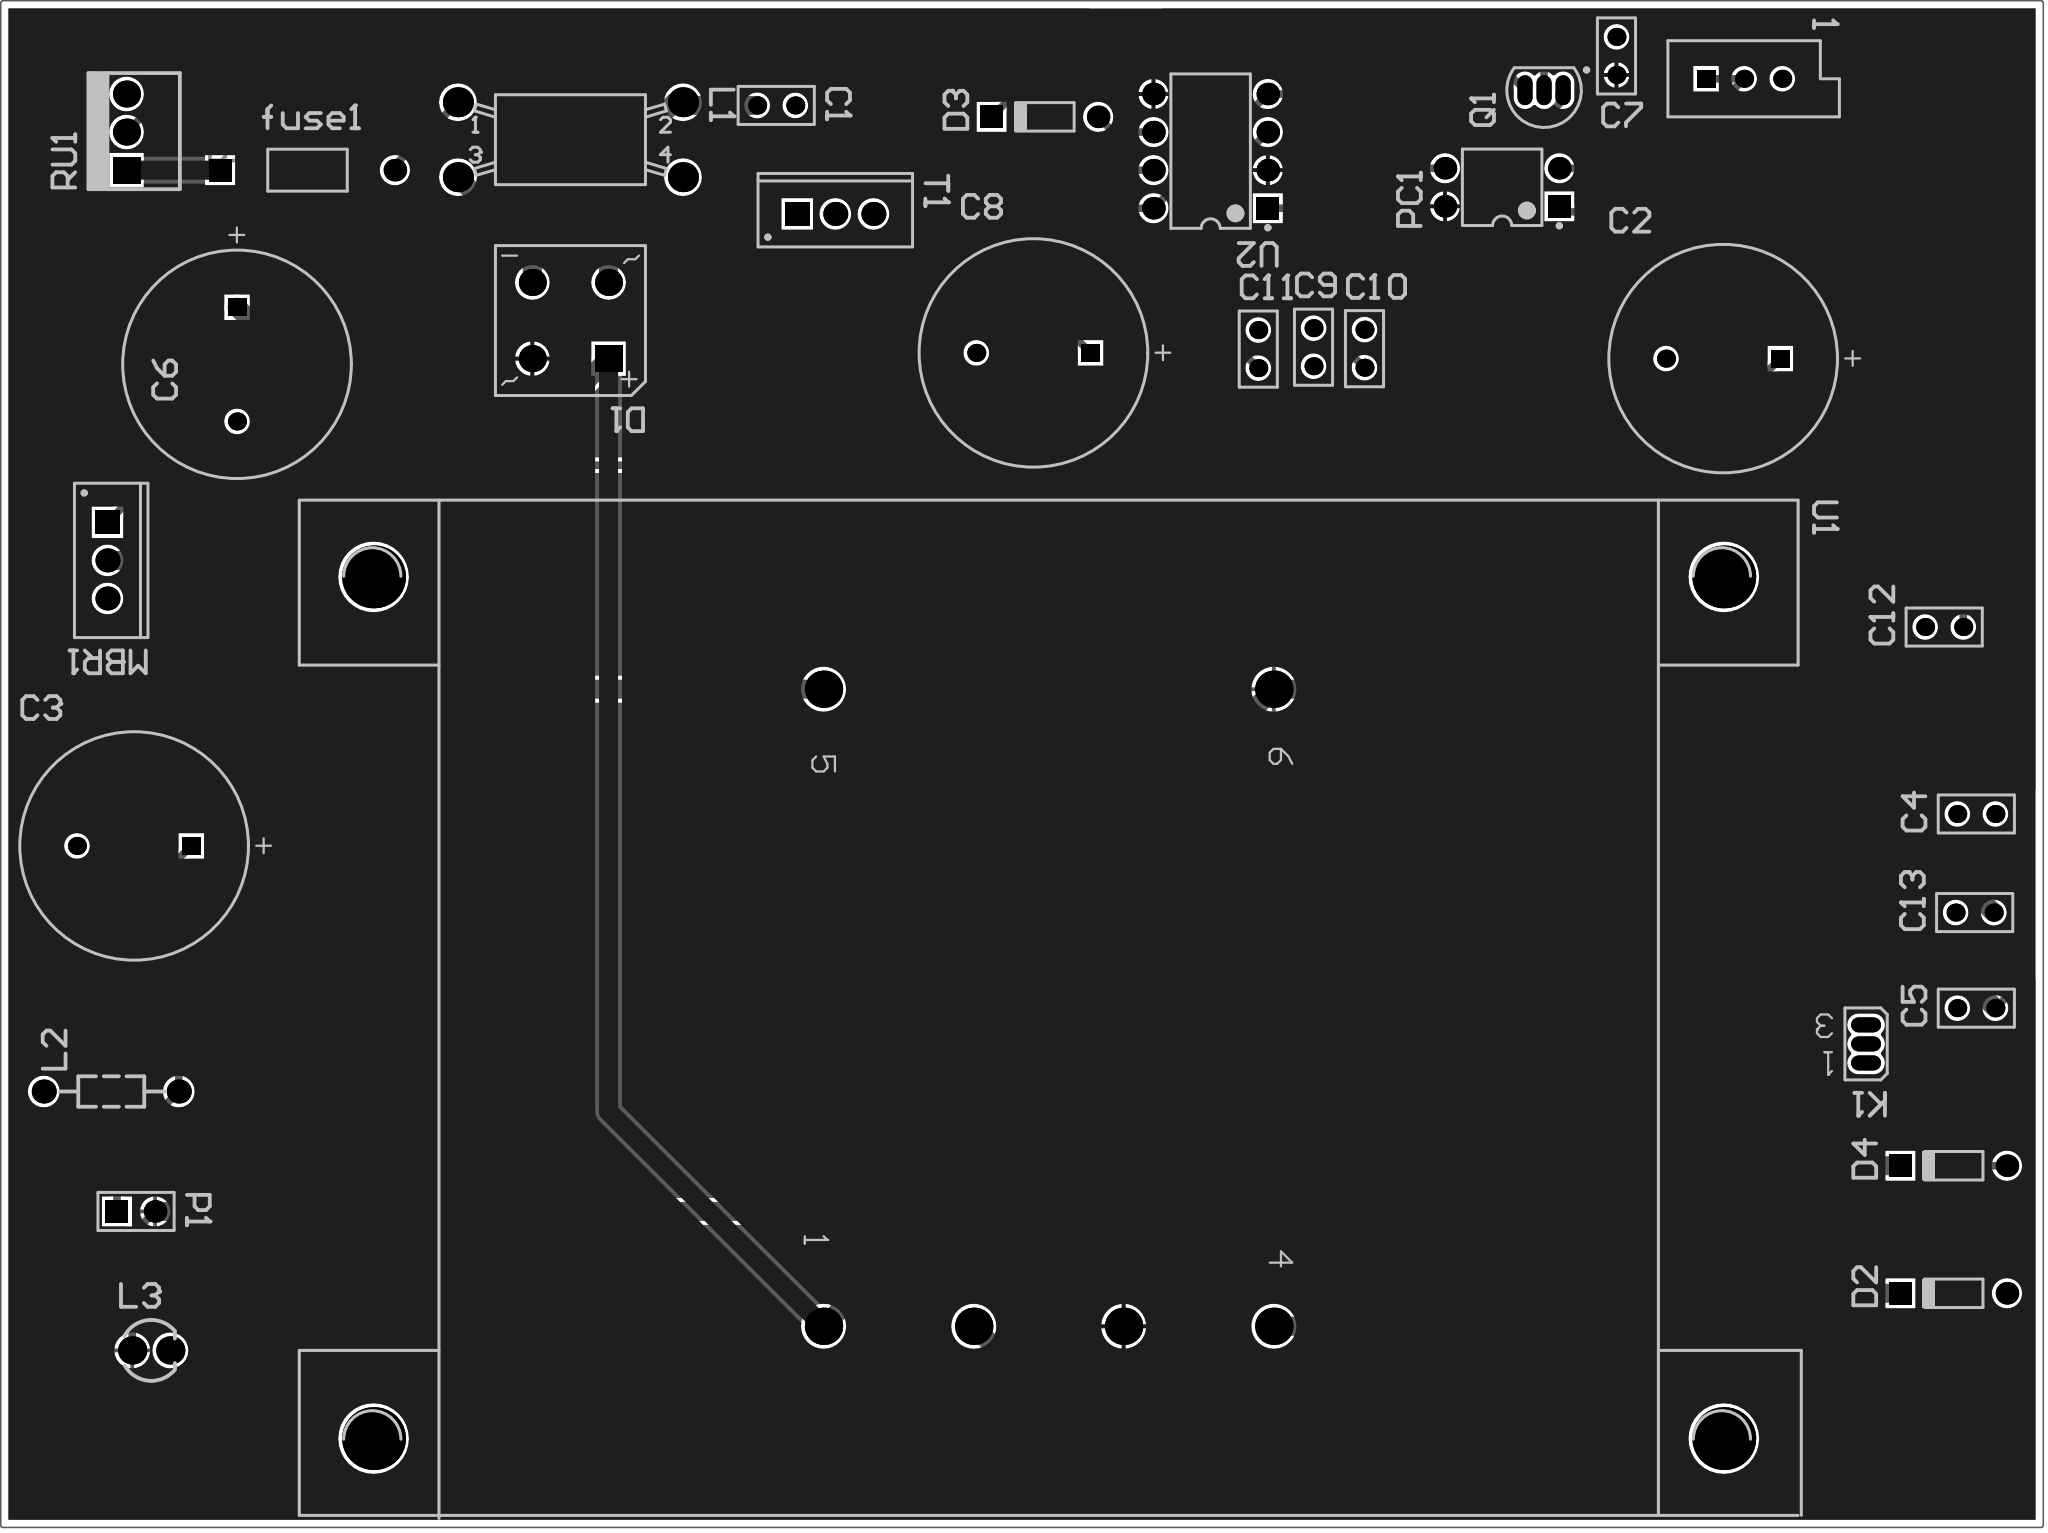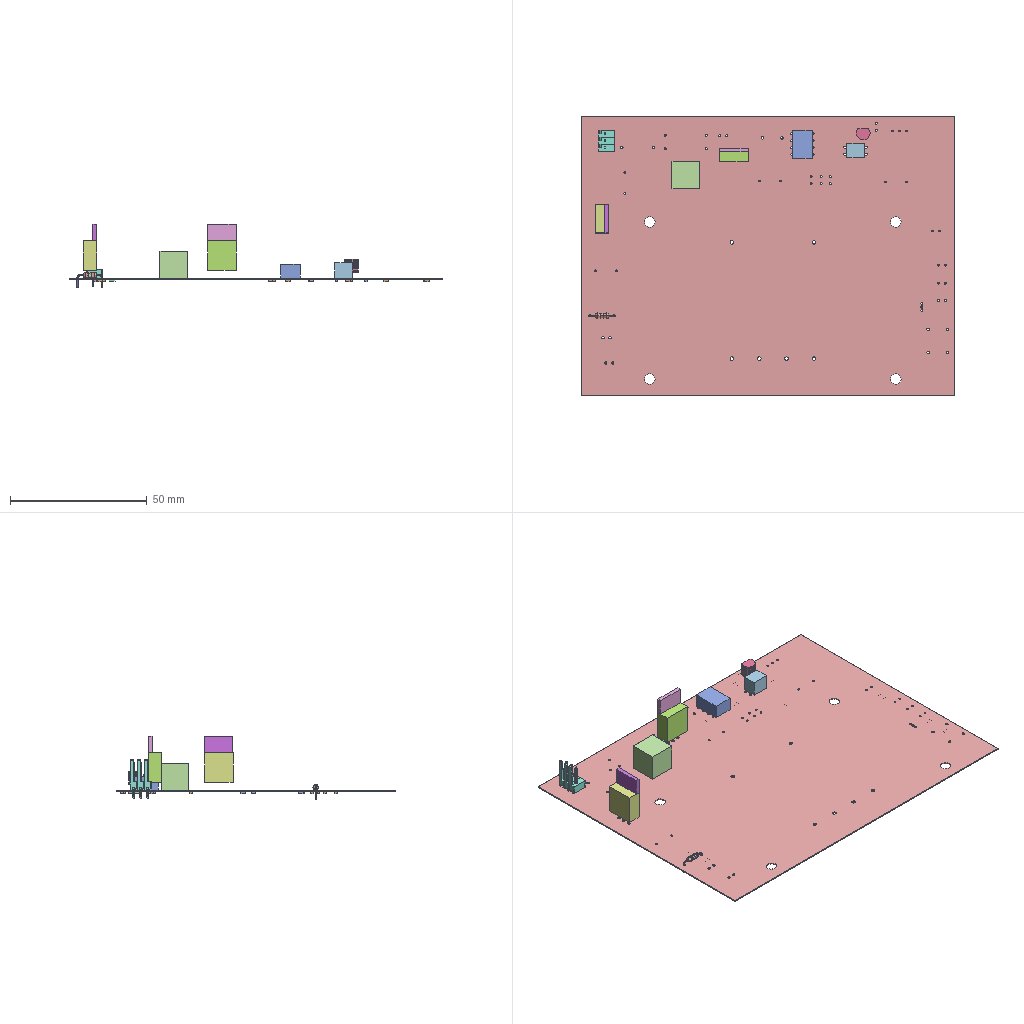Circuit board layout | Altium Designer | box 136.1 x 101.9 x 23.2 mm
Layer stack:
# Altium Designer layer stack of  (unit mm; dielectric type: 0 none, 1 core, 2 prepreg, 3 surface material)
index,name,kind,layer,copper_thickness_mm,dielectric_type,dielectric_thickness_mm,dielectric_material,dielectric_constant
0,Top Paste,other,,,,,,
1,Top Overlay,other,,,,,,
2,Top Solder,dielectric,,,3,0.0102,Solder Resist,3.5
3,Top Layer,copper,Top Layer,0.0356,,,,
4,Dielectric 1,dielectric,,,0,0.32,FR-4,4.8
5,Bottom Layer,copper,Bottom Layer,0.0356,,,,
6,Bottom Solder,dielectric,,,3,0.0102,Solder Resist,3.5
7,Bottom Overlay,other,,,,,,
8,Bottom Paste,other,,,,,,
# drill layer pairs: low layer,high layer
drill_pair,Top Layer,Bottom Layer
Part placement:
Designator,Comment,Layer,Footprint,Center-X(mm),Center-Y(mm),Rotation
U2,UC3842,TopLayer,DIP-8,113.538,135.255,180
U1,Transformer 1,TopLayer,TRF_6,102.743,78.105,270
T1,TL431,TopLayer,TO-262-AA,88.519,131.064,360
RU1,*,TopLayer,KF2510-3P,41.275,136.525,90
R19,2W 0.62,BottomLayer,J1-0603,163.703,71.501,0
R18,2K2,BottomLayer,J1-0603,148.602,133.477,0
R17,1W 10,BottomLayer,J1-0603,163.449,65.024,0
R16,1K,BottomLayer,J1-0603,112.649,142.494,0
R15,18K,BottomLayer,J1-0603,121.158,139.065,360
R14,470,BottomLayer,J1-0603,163.588,73.914,0
R13,15,BottomLayer,J1-0603,107.2,142.494,180
R12,470,BottomLayer,J1-0603,141.097,131.953,90
R11,20K,BottomLayer,J1-0603,43.942,69.088,0
R10,4K1,BottomLayer,J1-0603,121.285,131.445,360
R9,680,BottomLayer,J1-0603,106.299,131.445,180
R8,4K1,BottomLayer,J1-0603,135.763,142.99,90
R7,NTC 5D-11,BottomLayer,6-0805_N,48.376,137.922,360
R6,68k,BottomLayer,J1-0603,130.429,140.196,270
R5,10/1W,BottomLayer,J1-0603,134.505,118.11,180
R4,2K2,BottomLayer,J1-0603,42.037,77.978,90
R3,2W 330,BottomLayer,J1-0603,45.212,77.216,360
R2,2W 200K,BottomLayer,J1-0603,162.543,99.033,90
R1,2W 150K,BottomLayer,J1-0603,162.543,95.223,90
Q1,S8550,TopLayer,TO-92A,135.763,139.319,90
PC1,*,TopLayer,DIP-4,132.969,132.842,180
P1,Output,TopLayer,HDR1X2,41.91,64.516,360
MBR1,,TopLayer,TO-262-AA,40.005,107.95,270
L3,LED,TopLayer,LED3MM,42.926,55.245,0
L2,100UH,TopLayer,AL0204,40.259,72.517,180
L1,Filter,TopLayer,TRANS,70.866,136.017,360
K1,20N60,TopLayer,E3,157.226,75.692,180
fuse1,,TopLayer,PIN-W2/E2.8,53.34,133.985,360
D4,FR107,TopLayer,DO-35,163.068,67.564,180
D3,IN4148,TopLayer,DO-35,102.489,137.541,180
D2,FR107,TopLayer,DO-35,163.068,59.055,180
D1,1N4007*4,TopLayer,D-38,70.866,123.952,180
C13,104,TopLayer,RAD-0.1,164.465,84.455,180
C12,104,TopLayer,RAD-0.1,162.433,103.505,180
C11,222,TopLayer,RAD-0.1,116.713,122.047,90
C10,471,TopLayer,RAD-0.1,123.794,122.074,90
C9,225,TopLayer,RAD-0.1,120.396,122.174,90
C8,35V100U,TopLayer,RB7.6-15,101.727,121.793,0
C7,104,TopLayer,RAD-0.1,140.589,141.605,90
C6,400V  82uF,TopLayer,RB7.6-15,48.641,121.031,90
C5,222/2KV,TopLayer,RAD-0.1,164.575,78.078,180
C4,2KV 103,TopLayer,RAD-0.1,164.575,91.032,180
C3,35V 1000U,TopLayer,RB7.6-15,41.783,88.9,0
C2,35V 1000U,TopLayer,RB7.6-15,147.701,121.412,0
C1,0.1u 275V,TopLayer,RAD-0.1,84.582,138.303,360
1,,TopLayer,VR5,149.098,140.081,360
Pad and via stacks:
# Altium Designer via and pad stacks of  (unit mm). Each distinct definition once, with the count of objects using it.
# via: kind,start_layer,end_layer,hole_mm,diameter_mm,mode(0 simple;1 top-mid-bottom;2 full stack),diameter_per_layer,count,example_net
# pad: kind,layer,hole_mm,hole_type(0 round;1 square;2 slot),plating,top_size,top_shape(1 round;2 rect;3 octagon;9 rounded rect),mid_size,bottom_size,mode,footprint,size_per_layer,count,example
pad,Multi-Layer,1.2,0,plated,1.8x1.8,2,1.8x1.8,1.8x1.8,0,D-38,,1,D1.1
pad,Multi-Layer,1.2,0,plated,1.8x1.8,1,1.8x1.8,1.8x1.8,0,D-38,,3,D1.4
pad,Multi-Layer,0.9,0,plated,1.5x1.5,2,1.5x1.5,1.5x1.5,0,HDR1X2,,1,P1.1
pad,Multi-Layer,0.9,0,plated,1.5x1.5,1,1.5x1.5,1.5x1.5,0,HDR1X2,,1,P1.2
pad,Multi-Layer,1,0,plated,1.6x1.6,1,1.6x1.6,1.6x1.6,0,TO-262-AA,,4,MBR1.3
pad,Multi-Layer,1,0,plated,1.6x1.6,2,1.6x1.6,1.6x1.6,0,TO-262-AA,,2,MBR1.1
pad,Multi-Layer,0.8,0,plated,2x2,1,2x2,2x2,0,TRANS,,4,L1.1
pad,Multi-Layer,0.9,0,plated,1.5x1.5,1,1.5x1.5,1.5x1.5,0,PIN-W2/E2.8,,1,fuse1.2
pad,Multi-Layer,0.9,0,plated,1.5x1.5,2,1.5x1.5,1.5x1.5,0,PIN-W2/E2.8,,1,fuse1.1
pad,Multi-Layer,0.8,0,plated,1.6x1.6,1,1.6x1.6,1.6x1.6,0,AL0204,,2,L2.2
pad,Multi-Layer,1,0,plated,1.8x1.8,1,1.8x1.8,1.8x1.8,0,KF2510-3P,,2,RU1.3
pad,Multi-Layer,1,0,plated,1.8x1.8,2,1.8x1.8,1.8x1.8,0,KF2510-3P,,1,RU1.1
pad,Multi-Layer,1.321,0,plated,2.489x2.489,1,2.489x2.489,2.489x2.489,0,TRF_6,,6,U1.1
pad,Multi-Layer,3.861,0,plated,4.191x4.191,1,4.191x4.191,4.191x4.191,0,TRF_6,,4,U1.MH1
pad,Multi-Layer,0.7,0,plated,1.2x1.2,1,1.2x1.2,1.2x1.2,0,RAD-0.1,,18,C1.1
pad,Multi-Layer,0.7,0,plated,1.2x1.2,2,1.2x1.2,1.2x1.2,0,RB7.6-15,,4,C3.1
pad,Multi-Layer,0.7,0,plated,1.2x1.2,1,1.2x1.2,1.2x1.2,0,RB7.6-15,,4,C3.2
pad,Multi-Layer,0.8128,2,plated,1.88x1.88,1,1.88x1.88,1.88x1.88,0,LED3MM,,2,L3.2
pad,Multi-Layer,0.9,0,plated,2x1,1,2x1,2x1,0,TO-92A,,3,Q1.3
pad,Multi-Layer,0.9,0,plated,1.5x1.5,2,1.5x1.5,1.5x1.5,0,DO-35,,3,D2.2
pad,Multi-Layer,0.9,0,plated,1.5x1.5,1,1.5x1.5,1.5x1.5,0,DO-35,,3,D2.1
pad,Multi-Layer,0.9,0,plated,1.5x1.5,2,1.5x1.5,1.5x1.5,0,DIP-8,,1,U2.1
pad,Multi-Layer,0.9,0,plated,1.5x1.5,1,1.5x1.5,1.5x1.5,0,DIP-8,,7,U2.2
pad,Multi-Layer,0.8,0,plated,2x1,1,2x1,2x1,0,E3,,3,K1.1
pad,Multi-Layer,0.9,0,plated,1.5x1.5,1,1.5x1.5,1.5x1.5,0,DIP-4,,3,PC1.3
pad,Multi-Layer,0.9,0,plated,1.5x1.5,2,1.5x1.5,1.5x1.5,0,DIP-4,,1,PC1.1
pad,Multi-Layer,0.7,0,plated,1.2x1.2,2,1.2x1.2,1.2x1.2,0,VR5,,1,1.1
pad,Multi-Layer,0.7,0,plated,1.2x1.2,1,1.2x1.2,1.2x1.2,0,VR5,,2,1.2
pad,Bottom Layer,0,0,plated,0.9x0.7,2,0.9x0.7,0.9x0.7,0,J1-0603,,36,R4.1
pad,Bottom Layer,0,0,plated,1.4x1.2,2,1.4x1.2,1.4x1.2,0,6-0805_N,,2,R7.1
Copper pours:
name,layer,net,type(0 solid;1 hatched;2 none)
G,Bottom Layer,GND,0
G,Top Layer,GND,0
Design rules, without the lines most boards share:
# Altium Designer design rules of  (exported by Altium Designer, unit mm)
# columns: name | kind | enabled | priority | scope1 | scope2 | descriptor | typed fields (field=value)
SilkToSilkClearance | 55 | enabled | 1 | All | All | Silk to Silk (Clearance=0mil) (All),(All) |
SilkToSolderMaskClearance | 54 | enabled | 1 | IsPad | All | Silk To Solder Mask (Clearance=0mil) (IsPad),(All) |
MinimumSolderMaskSliver | 53 | enabled | 1 | All | All | Minimum Solder Mask Sliver (Gap=0mil) (All),(All) |
HoleToHoleClearance | 52 | enabled | 1 | All | All | Hole To Hole Clearance (Gap=10mil) (All),(All) | gap=0.254
DiffPairsRouting | 51 | enabled | 1 | All | All | Differential Pairs Uncoupled Length using the Gap Constraints (Min=10mil) (Max=10mil) (Prefered=10mil)  and Width Constraints (Min=15mil) (Max=15mil) (Prefered=15mil) (All) |
SolderMaskExpansion | 13 | enabled | 1 | All | All | Solder Mask Expansion (Expansion =4mil) (All) | expansion=0.1016
PasteMaskExpansion | 14 | enabled | 1 | All | All | Paste Mask Expansion (Expansion =0mil) (All) | expansion=0
RoutingVias | 11 | enabled | 1 | All | All | Routing Via (MinHoleWidth=28mil) (MaxHoleWidth=28mil) (PreferredHoleWidth=28mil) (MinWidth=50mil) (MaxWidth=50mil) (PreferedWidth=50mil) (All) | via_min_hole=0.7112 via_max_hole=0.7112 via_preferred_diameter=1.27 via_preferred_hole=0.7112
Width | 2 | enabled | 1 | All | All | Width Constraint (Min=10mil) (Max=70mil) (Preferred=10mil) (All) |
PolygonConnect | 20 | enabled | 1 | All | All | Polygon Connect Rule(Relief Connect )(Conductor Width=10mil) (Relief Angle=90 Angle) (Entries=4) (Air Gap Width=10mil) (All),(All) | connect_style(0=relief,1=direct,2=none)=0 relief_conductor_width=0.254 relief_entries=4
PlaneConnect | 6 | enabled | 1 | All | All | Power Plane Connect Rule(Relief Connect )(Expansion=20mil) (Conductor Width=10mil) (Air Gap=10mil) (Entries=4) (All) | relief_conductor_width=0.254 relief_entries=4 relief_expansion=0.508
Clearance | 0 | enabled | 1 | All | All | Clearance Constraint (Gap=10mil) (All),(All) | gap=0.254